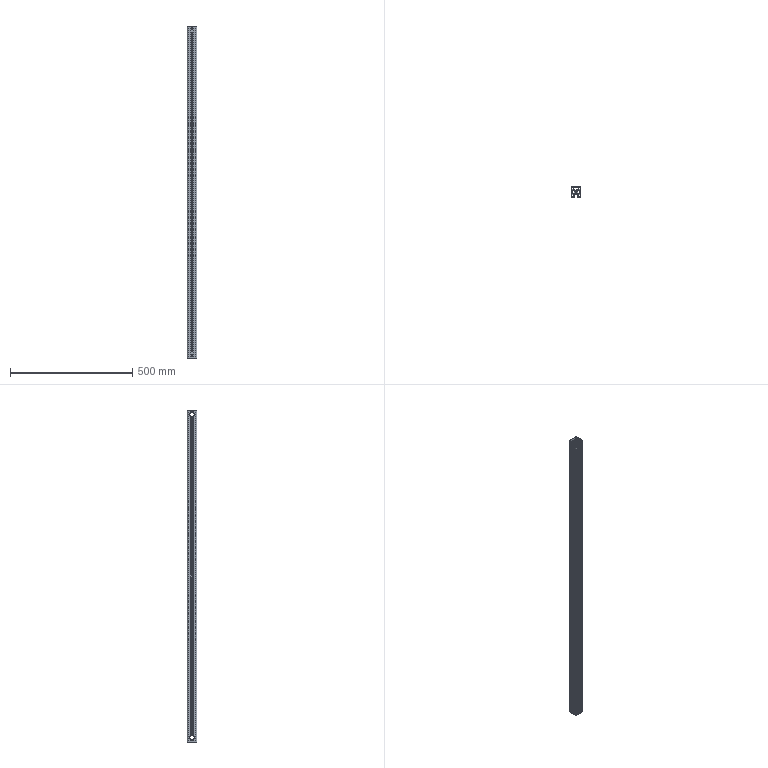Part | SolidWorks | features BaseBody 1, HoleWzd 1, MoveFace 1 | 1 solid | 242 faces | box 40 x 40 x 1360 mm | volume 796835 mm3 | plane 187 | cylinder 55 | commonest cylinder face diameters 6.8 x15 2 x14 19 x12 1 x6 5 x4 9 x4